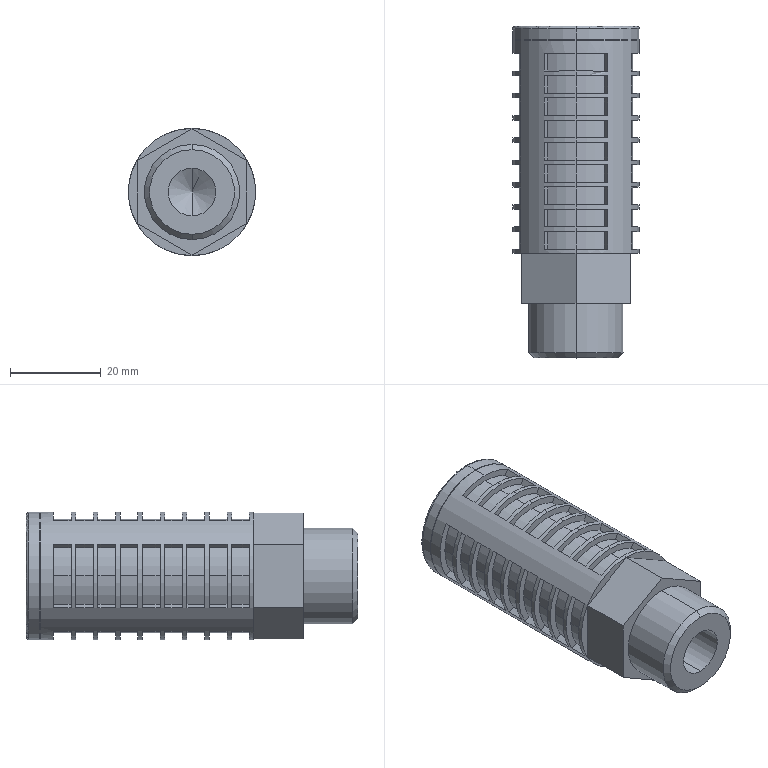Part | SolidWorks | features BaseBody 1 | 1 solid | 243 faces | box 28 x 73 x 28 mm | volume 31492 mm3 | plane 155 | cylinder 80 | cone 4 | torus 4 | commonest cylinder face diameters 25 x72 28 x4 10.478 x2 20.955 x2